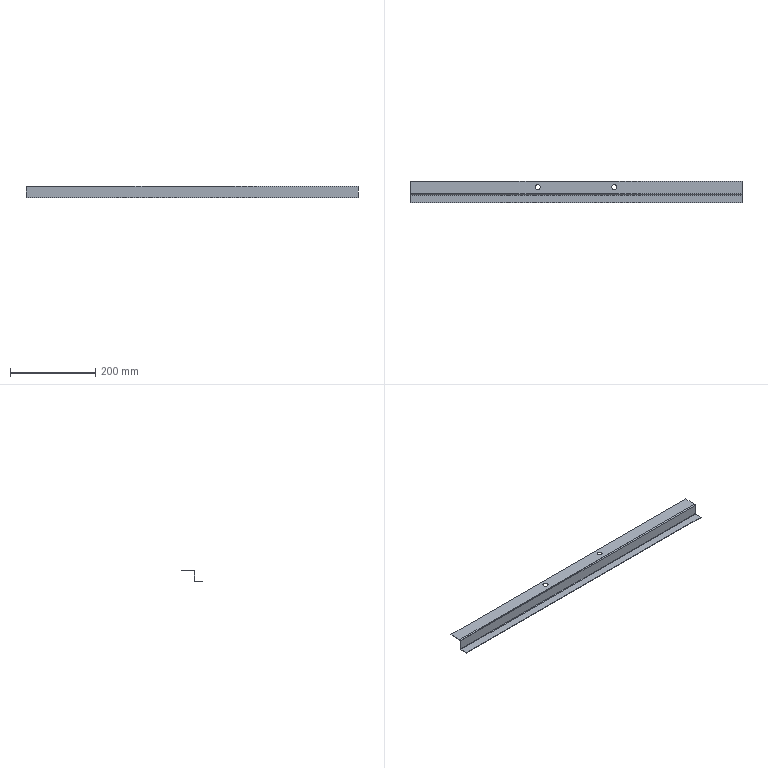Part | SolidWorks | features EdgeFlange 2, FlatPattern 1, HoleWzd 1, ICE 1, SMBaseFlange 1, SheetMetal 1 | 1 solid | 26 faces | box 780 x 50.8 x 28 mm | volume 71077 mm3 | plane 18 | cylinder 8 | commonest cylinder face diameters 12 x4 2 x2 4.4 x2
STEP:
#1=CARTESIAN_POINT('',(-84.,26.8,25.6));
#2=VERTEX_POINT('',#1);
#3=CARTESIAN_POINT('',(-96.,26.8,25.6));
#4=VERTEX_POINT('',#3);
#5=CARTESIAN_POINT('',(-90.,26.8,25.6));
#6=DIRECTION('',(0.,0.,-1.));
#7=DIRECTION('',(-1.,0.,0.));
#8=AXIS2_PLACEMENT_3D('',#5,#6,#7);
#9=CIRCLE('',#8,6.);
#10=EDGE_CURVE('',#2,#4,#9,.T.);
#11=ORIENTED_EDGE('',*,*,#10,.T.);
#12=CARTESIAN_POINT('',(-96.,26.8,26.8));
#13=VERTEX_POINT('',#12);
#14=CARTESIAN_POINT('',(-96.,26.8,16.8));
#15=DIRECTION('',(0.,0.,1.));
#16=VECTOR('',#15,1000.);
#17=LINE('',#14,#16);
#18=EDGE_CURVE('',#4,#13,#17,.T.);
#19=ORIENTED_EDGE('',*,*,#18,.T.);
#20=CARTESIAN_POINT('',(-84.,26.8,26.8));
#21=VERTEX_POINT('',#20);
#22=CARTESIAN_POINT('',(-90.,26.8,26.8));
#23=DIRECTION('',(0.,0.,1.));
#24=DIRECTION('',(1.,0.,0.));
#25=AXIS2_PLACEMENT_3D('',#22,#23,#24);
#26=CIRCLE('',#25,6.);
#27=EDGE_CURVE('',#13,#21,#26,.T.);
#28=ORIENTED_EDGE('',*,*,#27,.T.);
#29=CARTESIAN_POINT('',(-84.,26.8,16.8));
#30=DIRECTION('',(0.,0.,1.));
#31=VECTOR('',#30,1000.);
#32=LINE('',#29,#31);
#33=EDGE_CURVE('',#2,#21,#32,.T.);
#34=ORIENTED_EDGE('',*,*,#33,.F.);
#35=EDGE_LOOP('',(#11,#19,#28,#34));
#36=FACE_OUTER_BOUND('',#35,.T.);
#37=CARTESIAN_POINT('',(-90.,26.8,16.8));
#38=DIRECTION('',(0.,0.,1.));
#39=DIRECTION('',(1.,0.,0.));
#40=AXIS2_PLACEMENT_3D('',#37,#38,#39);
#41=CYLINDRICAL_SURFACE('',#40,6.);
#42=ADVANCED_FACE('',(#36),#41,.F.);
#43=CARTESIAN_POINT('',(96.,26.8,25.6));
#44=VERTEX_POINT('',#43);
#45=CARTESIAN_POINT('',(84.,26.8,25.6));
#46=VERTEX_POINT('',#45);
#47=CARTESIAN_POINT('',(90.,26.8,25.6));
#48=DIRECTION('',(0.,0.,-1.));
#49=DIRECTION('',(-1.,0.,0.));
#50=AXIS2_PLACEMENT_3D('',#47,#48,#49);
#51=CIRCLE('',#50,6.);
#52=EDGE_CURVE('',#44,#46,#51,.T.);
#53=ORIENTED_EDGE('',*,*,#52,.T.);
#54=CARTESIAN_POINT('',(84.,26.8,26.8));
#55=VERTEX_POINT('',#54);
#56=CARTESIAN_POINT('',(84.,26.8,16.8));
#57=DIRECTION('',(0.,0.,1.));
#58=VECTOR('',#57,1000.);
#59=LINE('',#56,#58);
#60=EDGE_CURVE('',#46,#55,#59,.T.);
#61=ORIENTED_EDGE('',*,*,#60,.T.);
#62=CARTESIAN_POINT('',(96.,26.8,26.8));
#63=VERTEX_POINT('',#62);
#64=CARTESIAN_POINT('',(90.,26.8,26.8));
#65=DIRECTION('',(0.,0.,1.));
#66=DIRECTION('',(-1.,0.,0.));
#67=AXIS2_PLACEMENT_3D('',#64,#65,#66);
#68=CIRCLE('',#67,6.);
#69=EDGE_CURVE('',#55,#63,#68,.T.);
#70=ORIENTED_EDGE('',*,*,#69,.T.);
#71=CARTESIAN_POINT('',(96.,26.8,16.8));
#72=DIRECTION('',(0.,0.,1.));
#73=VECTOR('',#72,1000.);
#74=LINE('',#71,#73);
#75=EDGE_CURVE('',#44,#63,#74,.T.);
#76=ORIENTED_EDGE('',*,*,#75,.F.);
#77=EDGE_LOOP('',(#53,#61,#70,#76));
#78=FACE_OUTER_BOUND('',#77,.T.);
#79=CARTESIAN_POINT('',(90.,26.8,16.8));
#80=DIRECTION('',(0.,0.,1.));
#81=DIRECTION('',(1.,0.,0.));
#82=AXIS2_PLACEMENT_3D('',#79,#80,#81);
#83=CYLINDRICAL_SURFACE('',#82,6.);
#84=ADVANCED_FACE('',(#78),#83,.F.);
#85=CARTESIAN_POINT('',(390.,10.,24.6));
#86=VERTEX_POINT('',#85);
#87=CARTESIAN_POINT('',(390.,8.8,24.6));
#88=VERTEX_POINT('',#87);
#89=CARTESIAN_POINT('',(390.,10.,24.6));
#90=DIRECTION('',(0.,-1.,0.));
#91=VECTOR('',#90,1000.);
#92=LINE('',#89,#91);
#93=EDGE_CURVE('',#86,#88,#92,.T.);
#94=ORIENTED_EDGE('',*,*,#93,.T.);
#95=CARTESIAN_POINT('',(390.,8.8,1.));
#96=VERTEX_POINT('',#95);
#97=CARTESIAN_POINT('',(390.,8.8,0.));
#98=DIRECTION('',(0.,0.,-1.));
#99=VECTOR('',#98,1000.);
#100=LINE('',#97,#99);
#101=EDGE_CURVE('',#88,#96,#100,.T.);
#102=ORIENTED_EDGE('',*,*,#101,.T.);
#103=CARTESIAN_POINT('',(390.,10.,1.));
#104=VERTEX_POINT('',#103);
#105=CARTESIAN_POINT('',(390.,10.,1.));
#106=DIRECTION('',(0.,1.,0.));
#107=VECTOR('',#106,1000.);
#108=LINE('',#105,#107);
#109=EDGE_CURVE('',#96,#104,#108,.T.);
#110=ORIENTED_EDGE('',*,*,#109,.T.);
#111=CARTESIAN_POINT('',(390.,10.,0.));
#112=DIRECTION('',(0.,0.,-1.));
#113=VECTOR('',#112,1000.);
#114=LINE('',#111,#113);
#115=EDGE_CURVE('',#86,#104,#114,.T.);
#116=ORIENTED_EDGE('',*,*,#115,.F.);
#117=EDGE_LOOP('',(#94,#102,#110,#116));
#118=FACE_OUTER_BOUND('',#117,.T.);
#119=CARTESIAN_POINT('',(390.,10.,0.));
#120=DIRECTION('',(-1.,0.,0.));
#121=DIRECTION('',(0.,0.,1.));
#122=AXIS2_PLACEMENT_3D('',#119,#120,#121);
#123=PLANE('',#122);
#124=ADVANCED_FACE('',(#118),#123,.F.);
#125=CARTESIAN_POINT('',(-390.,10.,24.6));
#126=VERTEX_POINT('',#125);
#127=CARTESIAN_POINT('',(-390.,8.8,24.6));
#128=VERTEX_POINT('',#127);
#129=CARTESIAN_POINT('',(-390.,10.,24.6));
#130=DIRECTION('',(0.,-1.,0.));
#131=VECTOR('',#130,1000.);
#132=LINE('',#129,#131);
#133=EDGE_CURVE('',#126,#128,#132,.T.);
#134=ORIENTED_EDGE('',*,*,#133,.F.);
#135=CARTESIAN_POINT('',(-390.,10.,1.));
#136=VERTEX_POINT('',#135);
#137=CARTESIAN_POINT('',(-390.,10.,0.));
#138=DIRECTION('',(0.,0.,1.));
#139=VECTOR('',#138,1000.);
#140=LINE('',#137,#139);
#141=EDGE_CURVE('',#136,#126,#140,.T.);
#142=ORIENTED_EDGE('',*,*,#141,.F.);
#143=CARTESIAN_POINT('',(-390.,8.8,1.));
#144=VERTEX_POINT('',#143);
#145=CARTESIAN_POINT('',(-390.,8.8,1.));
#146=DIRECTION('',(0.,1.,0.));
#147=VECTOR('',#146,1000.);
#148=LINE('',#145,#147);
#149=EDGE_CURVE('',#144,#136,#148,.T.);
#150=ORIENTED_EDGE('',*,*,#149,.F.);
#151=CARTESIAN_POINT('',(-390.,8.8,26.8));
#152=DIRECTION('',(0.,0.,1.));
#153=VECTOR('',#152,1000.);
#154=LINE('',#151,#153);
#155=EDGE_CURVE('',#144,#128,#154,.T.);
#156=ORIENTED_EDGE('',*,*,#155,.T.);
#157=EDGE_LOOP('',(#134,#142,#150,#156));
#158=FACE_OUTER_BOUND('',#157,.T.);
#159=CARTESIAN_POINT('',(-390.,10.,26.8));
#160=DIRECTION('',(1.,0.,0.));
#161=DIRECTION('',(0.,0.,-1.));
#162=AXIS2_PLACEMENT_3D('',#159,#160,#161);
#163=PLANE('',#162);
#164=ADVANCED_FACE('',(#158),#163,.F.);
#165=CARTESIAN_POINT('',(390.,10.,24.6));
#166=DIRECTION('',(-1.,0.,0.));
#167=VECTOR('',#166,1000.);
#168=LINE('',#165,#167);
#169=EDGE_CURVE('',#86,#126,#168,.T.);
#170=ORIENTED_EDGE('',*,*,#169,.F.);
#171=ORIENTED_EDGE('',*,*,#115,.T.);
#172=CARTESIAN_POINT('',(390.,10.,1.));
#173=DIRECTION('',(1.,0.,0.));
#174=VECTOR('',#173,1000.);
#175=LINE('',#172,#174);
#176=EDGE_CURVE('',#136,#104,#175,.T.);
#177=ORIENTED_EDGE('',*,*,#176,.F.);
#178=ORIENTED_EDGE('',*,*,#141,.T.);
#179=EDGE_LOOP('',(#170,#171,#177,#178));
#180=FACE_OUTER_BOUND('',#179,.T.);
#181=CARTESIAN_POINT('',(0.,10.,0.));
#182=DIRECTION('',(0.,-1.,0.));
#183=DIRECTION('',(0.,0.,-1.));
#184=AXIS2_PLACEMENT_3D('',#181,#182,#183);
#185=PLANE('',#184);
#186=ADVANCED_FACE('',(#180),#185,.F.);
#187=ORIENTED_EDGE('',*,*,#101,.F.);
#188=CARTESIAN_POINT('',(390.,8.8,24.6));
#189=DIRECTION('',(-1.,0.,0.));
#190=VECTOR('',#189,1000.);
#191=LINE('',#188,#190);
#192=EDGE_CURVE('',#88,#128,#191,.T.);
#193=ORIENTED_EDGE('',*,*,#192,.T.);
#194=ORIENTED_EDGE('',*,*,#155,.F.);
#195=CARTESIAN_POINT('',(390.,8.8,1.));
#196=DIRECTION('',(-1.,0.,0.));
#197=VECTOR('',#196,1000.);
#198=LINE('',#195,#197);
#199=EDGE_CURVE('',#96,#144,#198,.T.);
#200=ORIENTED_EDGE('',*,*,#199,.F.);
#201=EDGE_LOOP('',(#187,#193,#194,#200));
#202=FACE_OUTER_BOUND('',#201,.T.);
#203=CARTESIAN_POINT('',(0.,8.8,0.));
#204=DIRECTION('',(0.,-1.,0.));
#205=DIRECTION('',(0.,0.,-1.));
#206=AXIS2_PLACEMENT_3D('',#203,#204,#205);
#207=PLANE('',#206);
#208=ADVANCED_FACE('',(#202),#207,.T.);
#209=CARTESIAN_POINT('',(-390.,7.8,0.));
#210=VERTEX_POINT('',#209);
#211=CARTESIAN_POINT('',(-390.,-10.,0.));
#212=VERTEX_POINT('',#211);
#213=CARTESIAN_POINT('',(-390.,10.,0.));
#214=DIRECTION('',(0.,-1.,0.));
#215=VECTOR('',#214,1000.);
#216=LINE('',#213,#215);
#217=EDGE_CURVE('',#210,#212,#216,.T.);
#218=ORIENTED_EDGE('',*,*,#217,.F.);
#219=CARTESIAN_POINT('',(-390.,7.8,-1.2));
#220=VERTEX_POINT('',#219);
#221=CARTESIAN_POINT('',(-390.,7.8,0.));
#222=DIRECTION('',(0.,0.,-1.));
#223=VECTOR('',#222,1000.);
#224=LINE('',#221,#223);
#225=EDGE_CURVE('',#210,#220,#224,.T.);
#226=ORIENTED_EDGE('',*,*,#225,.T.);
#227=CARTESIAN_POINT('',(-390.,-10.,-1.2));
#228=VERTEX_POINT('',#227);
#229=CARTESIAN_POINT('',(-390.,10.,-1.2));
#230=DIRECTION('',(0.,-1.,0.));
#231=VECTOR('',#230,1000.);
#232=LINE('',#229,#231);
#233=EDGE_CURVE('',#220,#228,#232,.T.);
#234=ORIENTED_EDGE('',*,*,#233,.T.);
#235=CARTESIAN_POINT('',(-390.,-10.,-1.2));
#236=DIRECTION('',(0.,0.,1.));
#237=VECTOR('',#236,1000.);
#238=LINE('',#235,#237);
#239=EDGE_CURVE('',#228,#212,#238,.T.);
#240=ORIENTED_EDGE('',*,*,#239,.T.);
#241=EDGE_LOOP('',(#218,#226,#234,#240));
#242=FACE_OUTER_BOUND('',#241,.T.);
#243=CARTESIAN_POINT('',(-390.,10.,-1.2));
#244=DIRECTION('',(-1.,0.,0.));
#245=DIRECTION('',(0.,0.,1.));
#246=AXIS2_PLACEMENT_3D('',#243,#244,#245);
#247=PLANE('',#246);
#248=ADVANCED_FACE('',(#242),#247,.T.);
#249=CARTESIAN_POINT('',(390.,7.8,-1.2));
#250=VERTEX_POINT('',#249);
#251=CARTESIAN_POINT('',(-390.,7.8,-1.2));
#252=DIRECTION('',(1.,0.,0.));
#253=VECTOR('',#252,1000.);
#254=LINE('',#251,#253);
#255=EDGE_CURVE('',#220,#250,#254,.T.);
#256=ORIENTED_EDGE('',*,*,#255,.T.);
#257=CARTESIAN_POINT('',(390.,-10.,-1.2));
#258=VERTEX_POINT('',#257);
#259=CARTESIAN_POINT('',(390.,10.,-1.2));
#260=DIRECTION('',(0.,1.,0.));
#261=VECTOR('',#260,1000.);
#262=LINE('',#259,#261);
#263=EDGE_CURVE('',#258,#250,#262,.T.);
#264=ORIENTED_EDGE('',*,*,#263,.F.);
#265=CARTESIAN_POINT('',(-390.,-10.,-1.2));
#266=DIRECTION('',(1.,0.,0.));
#267=VECTOR('',#266,1000.);
#268=LINE('',#265,#267);
#269=EDGE_CURVE('',#228,#258,#268,.T.);
#270=ORIENTED_EDGE('',*,*,#269,.F.);
#271=ORIENTED_EDGE('',*,*,#233,.F.);
#272=EDGE_LOOP('',(#256,#264,#270,#271));
#273=FACE_OUTER_BOUND('',#272,.T.);
#274=CARTESIAN_POINT('',(0.,0.,-1.2));
#275=DIRECTION('',(0.,0.,1.));
#276=DIRECTION('',(1.,0.,0.));
#277=AXIS2_PLACEMENT_3D('',#274,#275,#276);
#278=PLANE('',#277);
#279=ADVANCED_FACE('',(#273),#278,.F.);
#280=CARTESIAN_POINT('',(390.,-10.,0.));
#281=VERTEX_POINT('',#280);
#282=CARTESIAN_POINT('',(390.,7.8,0.));
#283=VERTEX_POINT('',#282);
#284=CARTESIAN_POINT('',(390.,10.,0.));
#285=DIRECTION('',(0.,1.,0.));
#286=VECTOR('',#285,1000.);
#287=LINE('',#284,#286);
#288=EDGE_CURVE('',#281,#283,#287,.T.);
#289=ORIENTED_EDGE('',*,*,#288,.T.);
#290=CARTESIAN_POINT('',(-390.,7.8,0.));
#291=DIRECTION('',(1.,0.,0.));
#292=VECTOR('',#291,1000.);
#293=LINE('',#290,#292);
#294=EDGE_CURVE('',#210,#283,#293,.T.);
#295=ORIENTED_EDGE('',*,*,#294,.F.);
#296=ORIENTED_EDGE('',*,*,#217,.T.);
#297=CARTESIAN_POINT('',(-390.,-10.,0.));
#298=DIRECTION('',(1.,0.,0.));
#299=VECTOR('',#298,1000.);
#300=LINE('',#297,#299);
#301=EDGE_CURVE('',#212,#281,#300,.T.);
#302=ORIENTED_EDGE('',*,*,#301,.T.);
#303=EDGE_LOOP('',(#289,#295,#296,#302));
#304=FACE_OUTER_BOUND('',#303,.T.);
#305=CARTESIAN_POINT('',(0.,0.,0.));
#306=DIRECTION('',(0.,0.,1.));
#307=DIRECTION('',(1.,0.,0.));
#308=AXIS2_PLACEMENT_3D('',#305,#306,#307);
#309=PLANE('',#308);
#310=ADVANCED_FACE('',(#304),#309,.T.);
#311=CARTESIAN_POINT('',(390.,7.8,0.));
#312=DIRECTION('',(0.,0.,-1.));
#313=VECTOR('',#312,1000.);
#314=LINE('',#311,#313);
#315=EDGE_CURVE('',#283,#250,#314,.T.);
#316=ORIENTED_EDGE('',*,*,#315,.F.);
#317=ORIENTED_EDGE('',*,*,#288,.F.);
#318=CARTESIAN_POINT('',(390.,-10.,-1.2));
#319=DIRECTION('',(0.,0.,1.));
#320=VECTOR('',#319,1000.);
#321=LINE('',#318,#320);
#322=EDGE_CURVE('',#258,#281,#321,.T.);
#323=ORIENTED_EDGE('',*,*,#322,.F.);
#324=ORIENTED_EDGE('',*,*,#263,.T.);
#325=EDGE_LOOP('',(#316,#317,#323,#324));
#326=FACE_OUTER_BOUND('',#325,.T.);
#327=CARTESIAN_POINT('',(390.,10.,-1.2));
#328=DIRECTION('',(1.,0.,0.));
#329=DIRECTION('',(0.,0.,-1.));
#330=AXIS2_PLACEMENT_3D('',#327,#328,#329);
#331=PLANE('',#330);
#332=ADVANCED_FACE('',(#326),#331,.T.);
#333=ORIENTED_EDGE('',*,*,#301,.F.);
#334=ORIENTED_EDGE('',*,*,#239,.F.);
#335=ORIENTED_EDGE('',*,*,#269,.T.);
#336=ORIENTED_EDGE('',*,*,#322,.T.);
#337=EDGE_LOOP('',(#333,#334,#335,#336));
#338=FACE_OUTER_BOUND('',#337,.T.);
#339=CARTESIAN_POINT('',(-390.,-10.,-1.2));
#340=DIRECTION('',(0.,-1.,0.));
#341=DIRECTION('',(0.,0.,-1.));
#342=AXIS2_PLACEMENT_3D('',#339,#340,#341);
#343=PLANE('',#342);
#344=ADVANCED_FACE('',(#338),#343,.T.);
#345=ORIENTED_EDGE('',*,*,#109,.F.);
#346=CARTESIAN_POINT('',(390.,7.8,1.));
#347=DIRECTION('',(1.,0.,0.));
#348=DIRECTION('',(0.,0.,1.));
#349=AXIS2_PLACEMENT_3D('',#346,#347,#348);
#350=CIRCLE('',#349,1.);
#351=EDGE_CURVE('',#283,#96,#350,.T.);
#352=ORIENTED_EDGE('',*,*,#351,.F.);
#353=ORIENTED_EDGE('',*,*,#315,.T.);
#354=CARTESIAN_POINT('',(390.,7.8,1.));
#355=DIRECTION('',(1.,0.,0.));
#356=DIRECTION('',(0.,0.,1.));
#357=AXIS2_PLACEMENT_3D('',#354,#355,#356);
#358=CIRCLE('',#357,2.2);
#359=EDGE_CURVE('',#250,#104,#358,.T.);
#360=ORIENTED_EDGE('',*,*,#359,.T.);
#361=EDGE_LOOP('',(#345,#352,#353,#360));
#362=FACE_OUTER_BOUND('',#361,.T.);
#363=CARTESIAN_POINT('',(390.,7.8,1.));
#364=DIRECTION('',(1.,0.,0.));
#365=DIRECTION('',(0.,0.,-1.));
#366=AXIS2_PLACEMENT_3D('',#363,#364,#365);
#367=PLANE('',#366);
#368=ADVANCED_FACE('',(#362),#367,.T.);
#369=CARTESIAN_POINT('',(-390.,7.8,1.));
#370=DIRECTION('',(-1.,0.,0.));
#371=DIRECTION('',(0.,0.,1.));
#372=AXIS2_PLACEMENT_3D('',#369,#370,#371);
#373=CIRCLE('',#372,1.);
#374=EDGE_CURVE('',#144,#210,#373,.T.);
#375=ORIENTED_EDGE('',*,*,#374,.F.);
#376=ORIENTED_EDGE('',*,*,#149,.T.);
#377=CARTESIAN_POINT('',(-390.,7.8,1.));
#378=DIRECTION('',(-1.,0.,0.));
#379=DIRECTION('',(0.,0.,1.));
#380=AXIS2_PLACEMENT_3D('',#377,#378,#379);
#381=CIRCLE('',#380,2.2);
#382=EDGE_CURVE('',#136,#220,#381,.T.);
#383=ORIENTED_EDGE('',*,*,#382,.T.);
#384=ORIENTED_EDGE('',*,*,#225,.F.);
#385=EDGE_LOOP('',(#375,#376,#383,#384));
#386=FACE_OUTER_BOUND('',#385,.T.);
#387=CARTESIAN_POINT('',(-390.,7.8,1.));
#388=DIRECTION('',(1.,0.,0.));
#389=DIRECTION('',(0.,0.,-1.));
#390=AXIS2_PLACEMENT_3D('',#387,#388,#389);
#391=PLANE('',#390);
#392=ADVANCED_FACE('',(#386),#391,.F.);
#393=ORIENTED_EDGE('',*,*,#255,.F.);
#394=ORIENTED_EDGE('',*,*,#382,.F.);
#395=ORIENTED_EDGE('',*,*,#176,.T.);
#396=ORIENTED_EDGE('',*,*,#359,.F.);
#397=EDGE_LOOP('',(#393,#394,#395,#396));
#398=FACE_OUTER_BOUND('',#397,.T.);
#399=CARTESIAN_POINT('',(-390.,7.8,1.));
#400=DIRECTION('',(-1.,0.,0.));
#401=DIRECTION('',(0.,1.,0.));
#402=AXIS2_PLACEMENT_3D('',#399,#400,#401);
#403=CYLINDRICAL_SURFACE('',#402,2.2);
#404=ADVANCED_FACE('',(#398),#403,.T.);
#405=ORIENTED_EDGE('',*,*,#294,.T.);
#406=ORIENTED_EDGE('',*,*,#351,.T.);
#407=ORIENTED_EDGE('',*,*,#199,.T.);
#408=ORIENTED_EDGE('',*,*,#374,.T.);
#409=EDGE_LOOP('',(#405,#406,#407,#408));
#410=FACE_OUTER_BOUND('',#409,.T.);
#411=CARTESIAN_POINT('',(-390.,7.8,1.));
#412=DIRECTION('',(-1.,0.,0.));
#413=DIRECTION('',(0.,1.,0.));
#414=AXIS2_PLACEMENT_3D('',#411,#412,#413);
#415=CYLINDRICAL_SURFACE('',#414,1.);
#416=ADVANCED_FACE('',(#410),#415,.F.);
#417=CARTESIAN_POINT('',(-390.,11.,25.6));
#418=VERTEX_POINT('',#417);
#419=CARTESIAN_POINT('',(-390.,11.,26.8));
#420=VERTEX_POINT('',#419);
#421=CARTESIAN_POINT('',(-390.,11.,26.8));
#422=DIRECTION('',(0.,0.,1.));
#423=VECTOR('',#422,1000.);
#424=LINE('',#421,#423);
#425=EDGE_CURVE('',#418,#420,#424,.T.);
#426=ORIENTED_EDGE('',*,*,#425,.F.);
#427=CARTESIAN_POINT('',(-390.,11.,24.6));
#428=DIRECTION('',(-1.,0.,0.));
#429=DIRECTION('',(0.,0.,-1.));
#430=AXIS2_PLACEMENT_3D('',#427,#428,#429);
#431=CIRCLE('',#430,1.);
#432=EDGE_CURVE('',#126,#418,#431,.T.);
#433=ORIENTED_EDGE('',*,*,#432,.F.);
#434=ORIENTED_EDGE('',*,*,#133,.T.);
#435=CARTESIAN_POINT('',(-390.,11.,24.6));
#436=DIRECTION('',(-1.,0.,0.));
#437=DIRECTION('',(0.,0.,-1.));
#438=AXIS2_PLACEMENT_3D('',#435,#436,#437);
#439=CIRCLE('',#438,2.2);
#440=EDGE_CURVE('',#128,#420,#439,.T.);
#441=ORIENTED_EDGE('',*,*,#440,.T.);
#442=EDGE_LOOP('',(#426,#433,#434,#441));
#443=FACE_OUTER_BOUND('',#442,.T.);
#444=CARTESIAN_POINT('',(-390.,11.,24.6));
#445=DIRECTION('',(-1.,0.,0.));
#446=DIRECTION('',(0.,0.,1.));
#447=AXIS2_PLACEMENT_3D('',#444,#445,#446);
#448=PLANE('',#447);
#449=ADVANCED_FACE('',(#443),#448,.T.);
#450=CARTESIAN_POINT('',(390.,11.,25.6));
#451=VERTEX_POINT('',#450);
#452=CARTESIAN_POINT('',(390.,11.,24.6));
#453=DIRECTION('',(1.,0.,0.));
#454=DIRECTION('',(0.,0.,-1.));
#455=AXIS2_PLACEMENT_3D('',#452,#453,#454);
#456=CIRCLE('',#455,1.);
#457=EDGE_CURVE('',#451,#86,#456,.T.);
#458=ORIENTED_EDGE('',*,*,#457,.F.);
#459=CARTESIAN_POINT('',(390.,11.,26.8));
#460=VERTEX_POINT('',#459);
#461=CARTESIAN_POINT('',(390.,11.,25.6));
#462=DIRECTION('',(0.,0.,1.));
#463=VECTOR('',#462,1000.);
#464=LINE('',#461,#463);
#465=EDGE_CURVE('',#451,#460,#464,.T.);
#466=ORIENTED_EDGE('',*,*,#465,.T.);
#467=CARTESIAN_POINT('',(390.,11.,24.6));
#468=DIRECTION('',(1.,0.,0.));
#469=DIRECTION('',(0.,0.,-1.));
#470=AXIS2_PLACEMENT_3D('',#467,#468,#469);
#471=CIRCLE('',#470,2.2);
#472=EDGE_CURVE('',#460,#88,#471,.T.);
#473=ORIENTED_EDGE('',*,*,#472,.T.);
#474=ORIENTED_EDGE('',*,*,#93,.F.);
#475=EDGE_LOOP('',(#458,#466,#473,#474));
#476=FACE_OUTER_BOUND('',#475,.T.);
#477=CARTESIAN_POINT('',(390.,11.,24.6));
#478=DIRECTION('',(-1.,0.,0.));
#479=DIRECTION('',(0.,0.,1.));
#480=AXIS2_PLACEMENT_3D('',#477,#478,#479);
#481=PLANE('',#480);
#482=ADVANCED_FACE('',(#476),#481,.F.);
#483=ORIENTED_EDGE('',*,*,#192,.F.);
#484=ORIENTED_EDGE('',*,*,#472,.F.);
#485=CARTESIAN_POINT('',(-390.,11.,26.8));
#486=DIRECTION('',(-1.,0.,0.));
#487=VECTOR('',#486,1000.);
#488=LINE('',#485,#487);
#489=EDGE_CURVE('',#460,#420,#488,.T.);
#490=ORIENTED_EDGE('',*,*,#489,.T.);
#491=ORIENTED_EDGE('',*,*,#440,.F.);
#492=EDGE_LOOP('',(#483,#484,#490,#491));
#493=FACE_OUTER_BOUND('',#492,.T.);
#494=CARTESIAN_POINT('',(390.,11.,24.6));
#495=DIRECTION('',(1.,0.,0.));
#496=DIRECTION('',(0.,0.,1.));
#497=AXIS2_PLACEMENT_3D('',#494,#495,#496);
#498=CYLINDRICAL_SURFACE('',#497,2.2);
#499=ADVANCED_FACE('',(#493),#498,.T.);
#500=ORIENTED_EDGE('',*,*,#169,.T.);
#501=ORIENTED_EDGE('',*,*,#432,.T.);
#502=CARTESIAN_POINT('',(-390.,11.,25.6));
#503=DIRECTION('',(1.,0.,0.));
#504=VECTOR('',#503,1000.);
#505=LINE('',#502,#504);
#506=EDGE_CURVE('',#418,#451,#505,.T.);
#507=ORIENTED_EDGE('',*,*,#506,.T.);
#508=ORIENTED_EDGE('',*,*,#457,.T.);
#509=EDGE_LOOP('',(#500,#501,#507,#508));
#510=FACE_OUTER_BOUND('',#509,.T.);
#511=CARTESIAN_POINT('',(390.,11.,24.6));
#512=DIRECTION('',(1.,0.,0.));
#513=DIRECTION('',(0.,0.,1.));
#514=AXIS2_PLACEMENT_3D('',#511,#512,#513);
#515=CYLINDRICAL_SURFACE('',#514,1.);
#516=ADVANCED_FACE('',(#510),#515,.F.);
#517=ORIENTED_EDGE('',*,*,#425,.T.);
#518=CARTESIAN_POINT('',(-390.,40.8,26.8));
#519=VERTEX_POINT('',#518);
#520=CARTESIAN_POINT('',(-390.,0.,26.8));
#521=DIRECTION('',(0.,-1.,0.));
#522=VECTOR('',#521,1000.);
#523=LINE('',#520,#522);
#524=EDGE_CURVE('',#519,#420,#523,.T.);
#525=ORIENTED_EDGE('',*,*,#524,.F.);
#526=CARTESIAN_POINT('',(-390.,40.8,25.6));
#527=VERTEX_POINT('',#526);
#528=CARTESIAN_POINT('',(-390.,40.8,26.8));
#529=DIRECTION('',(0.,0.,-1.));
#530=VECTOR('',#529,1000.);
#531=LINE('',#528,#530);
#532=EDGE_CURVE('',#519,#527,#531,.T.);
#533=ORIENTED_EDGE('',*,*,#532,.T.);
#534=CARTESIAN_POINT('',(-390.,10.,25.6));
#535=DIRECTION('',(0.,-1.,0.));
#536=VECTOR('',#535,1000.);
#537=LINE('',#534,#536);
#538=EDGE_CURVE('',#527,#418,#537,.T.);
#539=ORIENTED_EDGE('',*,*,#538,.T.);
#540=EDGE_LOOP('',(#517,#525,#533,#539));
#541=FACE_OUTER_BOUND('',#540,.T.);
#542=CARTESIAN_POINT('',(-390.,10.,26.8));
#543=DIRECTION('',(1.,0.,0.));
#544=DIRECTION('',(0.,0.,-1.));
#545=AXIS2_PLACEMENT_3D('',#542,#543,#544);
#546=PLANE('',#545);
#547=ADVANCED_FACE('',(#541),#546,.F.);
#548=ORIENTED_EDGE('',*,*,#465,.F.);
#549=CARTESIAN_POINT('',(390.,40.8,25.6));
#550=VERTEX_POINT('',#549);
#551=CARTESIAN_POINT('',(390.,40.8,25.6));
#552=DIRECTION('',(0.,1.,0.));
#553=VECTOR('',#552,1000.);
#554=LINE('',#551,#553);
#555=EDGE_CURVE('',#451,#550,#554,.T.);
#556=ORIENTED_EDGE('',*,*,#555,.T.);
#557=CARTESIAN_POINT('',(390.,40.8,26.8));
#558=VERTEX_POINT('',#557);
#559=CARTESIAN_POINT('',(390.,40.8,26.8));
#560=DIRECTION('',(0.,0.,-1.));
#561=VECTOR('',#560,1000.);
#562=LINE('',#559,#561);
#563=EDGE_CURVE('',#558,#550,#562,.T.);
#564=ORIENTED_EDGE('',*,*,#563,.F.);
#565=CARTESIAN_POINT('',(390.,0.,26.8));
#566=DIRECTION('',(0.,1.,0.));
#567=VECTOR('',#566,1000.);
#568=LINE('',#565,#567);
#569=EDGE_CURVE('',#460,#558,#568,.T.);
#570=ORIENTED_EDGE('',*,*,#569,.F.);
#571=EDGE_LOOP('',(#548,#556,#564,#570));
#572=FACE_OUTER_BOUND('',#571,.T.);
#573=CARTESIAN_POINT('',(390.,40.8,26.8));
#574=DIRECTION('',(-1.,0.,0.));
#575=DIRECTION('',(0.,-1.,0.));
#576=AXIS2_PLACEMENT_3D('',#573,#574,#575);
#577=PLANE('',#576);
#578=ADVANCED_FACE('',(#572),#577,.F.);
#579=CARTESIAN_POINT('',(-90.,26.8,26.8));
#580=DIRECTION('',(0.,0.,1.));
#581=DIRECTION('',(1.,0.,0.));
#582=AXIS2_PLACEMENT_3D('',#579,#580,#581);
#583=CIRCLE('',#582,6.);
#584=EDGE_CURVE('',#21,#13,#583,.T.);
#585=ORIENTED_EDGE('',*,*,#584,.F.);
#586=ORIENTED_EDGE('',*,*,#27,.F.);
#587=EDGE_LOOP('',(#585,#586));
#588=FACE_BOUND('',#587,.T.);
#589=CARTESIAN_POINT('',(90.,26.8,26.8));
#590=DIRECTION('',(0.,0.,1.));
#591=DIRECTION('',(-1.,0.,0.));
#592=AXIS2_PLACEMENT_3D('',#589,#590,#591);
#593=CIRCLE('',#592,6.);
#594=EDGE_CURVE('',#63,#55,#593,.T.);
#595=ORIENTED_EDGE('',*,*,#594,.F.);
#596=ORIENTED_EDGE('',*,*,#69,.F.);
#597=EDGE_LOOP('',(#595,#596));
#598=FACE_BOUND('',#597,.T.);
#599=ORIENTED_EDGE('',*,*,#489,.F.);
#600=ORIENTED_EDGE('',*,*,#569,.T.);
#601=CARTESIAN_POINT('',(0.,40.8,26.8));
#602=DIRECTION('',(-1.,0.,0.));
#603=VECTOR('',#602,1000.);
#604=LINE('',#601,#603);
#605=EDGE_CURVE('',#558,#519,#604,.T.);
#606=ORIENTED_EDGE('',*,*,#605,.T.);
#607=ORIENTED_EDGE('',*,*,#524,.T.);
#608=EDGE_LOOP('',(#599,#600,#606,#607));
#609=FACE_OUTER_BOUND('',#608,.T.);
#610=CARTESIAN_POINT('',(0.,0.,26.8));
#611=DIRECTION('',(0.,0.,-1.));
#612=DIRECTION('',(-1.,0.,0.));
#613=AXIS2_PLACEMENT_3D('',#610,#611,#612);
#614=PLANE('',#613);
#615=ADVANCED_FACE('',(#588,#598,#609),#614,.F.);
#616=ORIENTED_EDGE('',*,*,#10,.F.);
#617=CARTESIAN_POINT('',(-90.,26.8,25.6));
#618=DIRECTION('',(0.,0.,-1.));
#619=DIRECTION('',(-1.,0.,0.));
#620=AXIS2_PLACEMENT_3D('',#617,#618,#619);
#621=CIRCLE('',#620,6.);
#622=EDGE_CURVE('',#4,#2,#621,.T.);
#623=ORIENTED_EDGE('',*,*,#622,.F.);
#624=EDGE_LOOP('',(#616,#623));
#625=FACE_BOUND('',#624,.T.);
#626=ORIENTED_EDGE('',*,*,#52,.F.);
#627=CARTESIAN_POINT('',(90.,26.8,25.6));
#628=DIRECTION('',(0.,0.,-1.));
#629=DIRECTION('',(-1.,0.,0.));
#630=AXIS2_PLACEMENT_3D('',#627,#628,#629);
#631=CIRCLE('',#630,6.);
#632=EDGE_CURVE('',#46,#44,#631,.T.);
#633=ORIENTED_EDGE('',*,*,#632,.F.);
#634=EDGE_LOOP('',(#626,#633));
#635=FACE_BOUND('',#634,.T.);
#636=ORIENTED_EDGE('',*,*,#555,.F.);
#637=ORIENTED_EDGE('',*,*,#506,.F.);
#638=ORIENTED_EDGE('',*,*,#538,.F.);
#639=CARTESIAN_POINT('',(-390.,40.8,25.6));
#640=DIRECTION('',(-1.,0.,0.));
#641=VECTOR('',#640,1000.);
#642=LINE('',#639,#641);
#643=EDGE_CURVE('',#550,#527,#642,.T.);
#644=ORIENTED_EDGE('',*,*,#643,.F.);
#645=EDGE_LOOP('',(#636,#637,#638,#644));
#646=FACE_OUTER_BOUND('',#645,.T.);
#647=CARTESIAN_POINT('',(0.,0.,25.6));
#648=DIRECTION('',(0.,0.,-1.));
#649=DIRECTION('',(-1.,0.,0.));
#650=AXIS2_PLACEMENT_3D('',#647,#648,#649);
#651=PLANE('',#650);
#652=ADVANCED_FACE('',(#625,#635,#646),#651,.T.);
#653=ORIENTED_EDGE('',*,*,#643,.T.);
#654=ORIENTED_EDGE('',*,*,#532,.F.);
#655=ORIENTED_EDGE('',*,*,#605,.F.);
#656=ORIENTED_EDGE('',*,*,#563,.T.);
#657=EDGE_LOOP('',(#653,#654,#655,#656));
#658=FACE_OUTER_BOUND('',#657,.T.);
#659=CARTESIAN_POINT('',(-390.,40.8,26.8));
#660=DIRECTION('',(0.,-1.,0.));
#661=DIRECTION('',(0.,0.,-1.));
#662=AXIS2_PLACEMENT_3D('',#659,#660,#661);
#663=PLANE('',#662);
#664=ADVANCED_FACE('',(#658),#663,.F.);
#665=ORIENTED_EDGE('',*,*,#60,.F.);
#666=ORIENTED_EDGE('',*,*,#632,.T.);
#667=ORIENTED_EDGE('',*,*,#75,.T.);
#668=ORIENTED_EDGE('',*,*,#594,.T.);
#669=EDGE_LOOP('',(#665,#666,#667,#668));
#670=FACE_OUTER_BOUND('',#669,.T.);
#671=CARTESIAN_POINT('',(90.,26.8,16.8));
#672=DIRECTION('',(0.,0.,1.));
#673=DIRECTION('',(1.,0.,0.));
#674=AXIS2_PLACEMENT_3D('',#671,#672,#673);
#675=CYLINDRICAL_SURFACE('',#674,6.);
#676=ADVANCED_FACE('',(#670),#675,.F.);
#677=ORIENTED_EDGE('',*,*,#18,.F.);
#678=ORIENTED_EDGE('',*,*,#622,.T.);
#679=ORIENTED_EDGE('',*,*,#33,.T.);
#680=ORIENTED_EDGE('',*,*,#584,.T.);
#681=EDGE_LOOP('',(#677,#678,#679,#680));
#682=FACE_OUTER_BOUND('',#681,.T.);
#683=CARTESIAN_POINT('',(-90.,26.8,16.8));
#684=DIRECTION('',(0.,0.,1.));
#685=DIRECTION('',(1.,0.,0.));
#686=AXIS2_PLACEMENT_3D('',#683,#684,#685);
#687=CYLINDRICAL_SURFACE('',#686,6.);
#688=ADVANCED_FACE('',(#682),#687,.F.);
#689=CLOSED_SHELL('',(#42,#84,#124,#164,#186,#208,#248,#279,#310,#332,#344,#368,#392,#404,#416,#449,#482,#499,#516,#547,#578,#615,#652,#664,#676,#688));
#690=MANIFOLD_SOLID_BREP('',#689);
#691=CARTESIAN_POINT('',(0.,0.,0.));
#692=DIRECTION('',(0.,0.,1.));
#693=DIRECTION('',(1.,0.,0.));
#694=AXIS2_PLACEMENT_3D('',#691,#692,#693);
#695=(LENGTH_UNIT()NAMED_UNIT(*)SI_UNIT(.MILLI.,.METRE.));
#696=UNCERTAINTY_MEASURE_WITH_UNIT(LENGTH_MEASURE(0.00001),#695,'','');
#697=(NAMED_UNIT(*)PLANE_ANGLE_UNIT()SI_UNIT($,.RADIAN.));
#698=(NAMED_UNIT(*)SI_UNIT($,.STERADIAN.)SOLID_ANGLE_UNIT());
#699=(GEOMETRIC_REPRESENTATION_CONTEXT(3)GLOBAL_UNCERTAINTY_ASSIGNED_CONTEXT((#696))GLOBAL_UNIT_ASSIGNED_CONTEXT((#695,#697,#698))REPRESENTATION_CONTEXT('',''));
#700=ADVANCED_BREP_SHAPE_REPRESENTATION('',(#690,#694),#699);